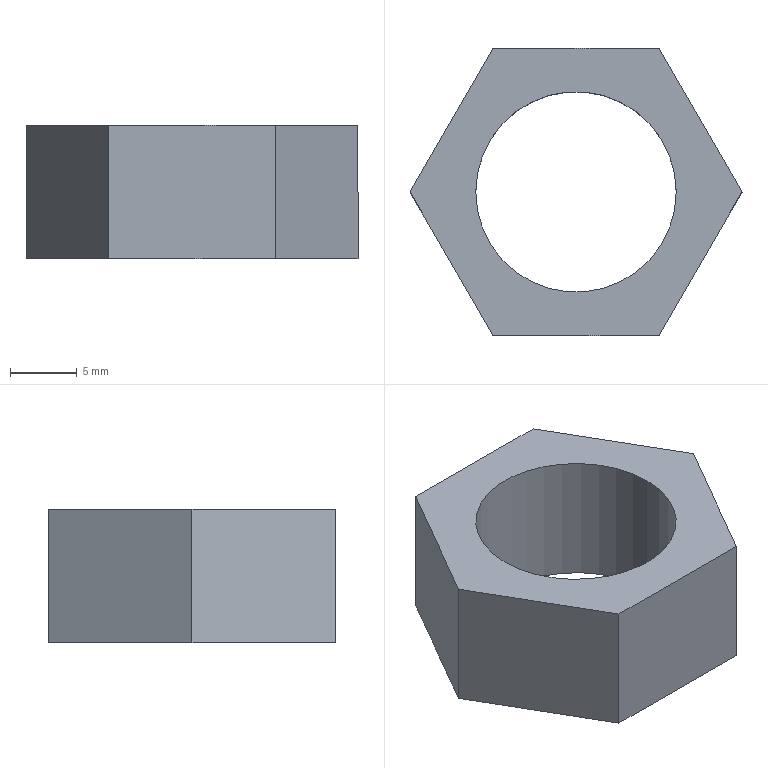Part | SolidWorks | features BaseBody 1 | 1 solid | 10 faces | box 24.848 x 21.519 x 10 mm | volume 2243 mm3 | plane 8 | cylinder 2 | commonest cylinder face diameters 15 x2
STEP:
#1=CARTESIAN_POINT('',(7.5,0.,0.));
#2=VERTEX_POINT('',#1);
#3=CARTESIAN_POINT('',(-7.5,0.,0.));
#4=VERTEX_POINT('',#3);
#5=CARTESIAN_POINT('',(0.,0.,0.));
#6=DIRECTION('',(0.,0.,-1.));
#7=DIRECTION('',(-1.,0.,0.));
#8=AXIS2_PLACEMENT_3D('',#5,#6,#7);
#9=CIRCLE('',#8,7.5);
#10=EDGE_CURVE('',#2,#4,#9,.T.);
#11=ORIENTED_EDGE('',*,*,#10,.F.);
#12=CARTESIAN_POINT('',(7.5,0.,-10.));
#13=VERTEX_POINT('',#12);
#14=CARTESIAN_POINT('',(7.5,0.,0.));
#15=DIRECTION('',(0.,0.,-1.));
#16=VECTOR('',#15,1000.);
#17=LINE('',#14,#16);
#18=EDGE_CURVE('',#2,#13,#17,.T.);
#19=ORIENTED_EDGE('',*,*,#18,.T.);
#20=CARTESIAN_POINT('',(-7.5,0.,-10.));
#21=VERTEX_POINT('',#20);
#22=CARTESIAN_POINT('',(0.,0.,-10.));
#23=DIRECTION('',(0.,0.,1.));
#24=DIRECTION('',(-1.,0.,0.));
#25=AXIS2_PLACEMENT_3D('',#22,#23,#24);
#26=CIRCLE('',#25,7.5);
#27=EDGE_CURVE('',#21,#13,#26,.T.);
#28=ORIENTED_EDGE('',*,*,#27,.F.);
#29=CARTESIAN_POINT('',(-7.5,0.,0.));
#30=DIRECTION('',(0.,0.,-1.));
#31=VECTOR('',#30,1000.);
#32=LINE('',#29,#31);
#33=EDGE_CURVE('',#4,#21,#32,.T.);
#34=ORIENTED_EDGE('',*,*,#33,.F.);
#35=EDGE_LOOP('',(#11,#19,#28,#34));
#36=FACE_OUTER_BOUND('',#35,.T.);
#37=CARTESIAN_POINT('',(0.,0.,0.));
#38=DIRECTION('',(0.,0.,-1.));
#39=DIRECTION('',(-1.,0.,0.));
#40=AXIS2_PLACEMENT_3D('',#37,#38,#39);
#41=CYLINDRICAL_SURFACE('',#40,7.5);
#42=ADVANCED_FACE('',(#36),#41,.F.);
#43=ORIENTED_EDGE('',*,*,#18,.F.);
#44=CARTESIAN_POINT('',(0.,0.,0.));
#45=DIRECTION('',(0.,0.,-1.));
#46=DIRECTION('',(-1.,0.,0.));
#47=AXIS2_PLACEMENT_3D('',#44,#45,#46);
#48=CIRCLE('',#47,7.5);
#49=EDGE_CURVE('',#4,#2,#48,.T.);
#50=ORIENTED_EDGE('',*,*,#49,.F.);
#51=ORIENTED_EDGE('',*,*,#33,.T.);
#52=CARTESIAN_POINT('',(0.,0.,-10.));
#53=DIRECTION('',(0.,0.,1.));
#54=DIRECTION('',(-1.,0.,0.));
#55=AXIS2_PLACEMENT_3D('',#52,#53,#54);
#56=CIRCLE('',#55,7.5);
#57=EDGE_CURVE('',#13,#21,#56,.T.);
#58=ORIENTED_EDGE('',*,*,#57,.F.);
#59=EDGE_LOOP('',(#43,#50,#51,#58));
#60=FACE_OUTER_BOUND('',#59,.T.);
#61=CARTESIAN_POINT('',(0.,0.,0.));
#62=DIRECTION('',(0.,0.,-1.));
#63=DIRECTION('',(-1.,0.,0.));
#64=AXIS2_PLACEMENT_3D('',#61,#62,#63);
#65=CYLINDRICAL_SURFACE('',#64,7.5);
#66=ADVANCED_FACE('',(#60),#65,.F.);
#67=ORIENTED_EDGE('',*,*,#27,.T.);
#68=ORIENTED_EDGE('',*,*,#57,.T.);
#69=EDGE_LOOP('',(#67,#68));
#70=FACE_BOUND('',#69,.T.);
#71=CARTESIAN_POINT('',(-6.212,-10.76,-10.));
#72=VERTEX_POINT('',#71);
#73=CARTESIAN_POINT('',(6.212,-10.76,-10.));
#74=VERTEX_POINT('',#73);
#75=CARTESIAN_POINT('',(0.,-10.76,-10.));
#76=DIRECTION('',(1.,0.,0.));
#77=VECTOR('',#76,1000.);
#78=LINE('',#75,#77);
#79=EDGE_CURVE('',#72,#74,#78,.T.);
#80=ORIENTED_EDGE('',*,*,#79,.F.);
#81=CARTESIAN_POINT('',(-12.424,0.,-10.));
#82=VERTEX_POINT('',#81);
#83=CARTESIAN_POINT('',(-12.424,0.,-10.));
#84=DIRECTION('',(0.5,-0.866,0.));
#85=VECTOR('',#84,1000.);
#86=LINE('',#83,#85);
#87=EDGE_CURVE('',#82,#72,#86,.T.);
#88=ORIENTED_EDGE('',*,*,#87,.F.);
#89=CARTESIAN_POINT('',(-6.212,10.76,-10.));
#90=VERTEX_POINT('',#89);
#91=CARTESIAN_POINT('',(-6.212,10.76,-10.));
#92=DIRECTION('',(-0.5,-0.866,0.));
#93=VECTOR('',#92,1000.);
#94=LINE('',#91,#93);
#95=EDGE_CURVE('',#90,#82,#94,.T.);
#96=ORIENTED_EDGE('',*,*,#95,.F.);
#97=CARTESIAN_POINT('',(6.212,10.76,-10.));
#98=VERTEX_POINT('',#97);
#99=CARTESIAN_POINT('',(0.,10.76,-10.));
#100=DIRECTION('',(-1.,0.,0.));
#101=VECTOR('',#100,1000.);
#102=LINE('',#99,#101);
#103=EDGE_CURVE('',#98,#90,#102,.T.);
#104=ORIENTED_EDGE('',*,*,#103,.F.);
#105=CARTESIAN_POINT('',(12.424,0.,-10.));
#106=VERTEX_POINT('',#105);
#107=CARTESIAN_POINT('',(12.424,0.,-10.));
#108=DIRECTION('',(-0.5,0.866,0.));
#109=VECTOR('',#108,1000.);
#110=LINE('',#107,#109);
#111=EDGE_CURVE('',#106,#98,#110,.T.);
#112=ORIENTED_EDGE('',*,*,#111,.F.);
#113=CARTESIAN_POINT('',(6.212,-10.76,-10.));
#114=DIRECTION('',(0.5,0.866,0.));
#115=VECTOR('',#114,1000.);
#116=LINE('',#113,#115);
#117=EDGE_CURVE('',#74,#106,#116,.T.);
#118=ORIENTED_EDGE('',*,*,#117,.F.);
#119=EDGE_LOOP('',(#80,#88,#96,#104,#112,#118));
#120=FACE_OUTER_BOUND('',#119,.T.);
#121=CARTESIAN_POINT('',(0.,0.,-10.));
#122=DIRECTION('',(0.,0.,1.));
#123=DIRECTION('',(1.,0.,0.));
#124=AXIS2_PLACEMENT_3D('',#121,#122,#123);
#125=PLANE('',#124);
#126=ADVANCED_FACE('',(#70,#120),#125,.F.);
#127=ORIENTED_EDGE('',*,*,#49,.T.);
#128=ORIENTED_EDGE('',*,*,#10,.T.);
#129=EDGE_LOOP('',(#127,#128));
#130=FACE_BOUND('',#129,.T.);
#131=CARTESIAN_POINT('',(-12.424,0.,0.));
#132=VERTEX_POINT('',#131);
#133=CARTESIAN_POINT('',(-6.212,-10.76,0.));
#134=VERTEX_POINT('',#133);
#135=CARTESIAN_POINT('',(-12.424,0.,0.));
#136=DIRECTION('',(0.5,-0.866,0.));
#137=VECTOR('',#136,1000.);
#138=LINE('',#135,#137);
#139=EDGE_CURVE('',#132,#134,#138,.T.);
#140=ORIENTED_EDGE('',*,*,#139,.T.);
#141=CARTESIAN_POINT('',(6.212,-10.76,0.));
#142=VERTEX_POINT('',#141);
#143=CARTESIAN_POINT('',(0.,-10.76,0.));
#144=DIRECTION('',(1.,0.,0.));
#145=VECTOR('',#144,1000.);
#146=LINE('',#143,#145);
#147=EDGE_CURVE('',#134,#142,#146,.T.);
#148=ORIENTED_EDGE('',*,*,#147,.T.);
#149=CARTESIAN_POINT('',(12.424,0.,0.));
#150=VERTEX_POINT('',#149);
#151=CARTESIAN_POINT('',(6.212,-10.76,0.));
#152=DIRECTION('',(0.5,0.866,0.));
#153=VECTOR('',#152,1000.);
#154=LINE('',#151,#153);
#155=EDGE_CURVE('',#142,#150,#154,.T.);
#156=ORIENTED_EDGE('',*,*,#155,.T.);
#157=CARTESIAN_POINT('',(6.212,10.76,0.));
#158=VERTEX_POINT('',#157);
#159=CARTESIAN_POINT('',(12.424,0.,0.));
#160=DIRECTION('',(-0.5,0.866,0.));
#161=VECTOR('',#160,1000.);
#162=LINE('',#159,#161);
#163=EDGE_CURVE('',#150,#158,#162,.T.);
#164=ORIENTED_EDGE('',*,*,#163,.T.);
#165=CARTESIAN_POINT('',(-6.212,10.76,0.));
#166=VERTEX_POINT('',#165);
#167=CARTESIAN_POINT('',(0.,10.76,0.));
#168=DIRECTION('',(-1.,0.,0.));
#169=VECTOR('',#168,1000.);
#170=LINE('',#167,#169);
#171=EDGE_CURVE('',#158,#166,#170,.T.);
#172=ORIENTED_EDGE('',*,*,#171,.T.);
#173=CARTESIAN_POINT('',(-6.212,10.76,0.));
#174=DIRECTION('',(-0.5,-0.866,0.));
#175=VECTOR('',#174,1000.);
#176=LINE('',#173,#175);
#177=EDGE_CURVE('',#166,#132,#176,.T.);
#178=ORIENTED_EDGE('',*,*,#177,.T.);
#179=EDGE_LOOP('',(#140,#148,#156,#164,#172,#178));
#180=FACE_OUTER_BOUND('',#179,.T.);
#181=CARTESIAN_POINT('',(0.,0.,0.));
#182=DIRECTION('',(0.,0.,1.));
#183=DIRECTION('',(1.,0.,0.));
#184=AXIS2_PLACEMENT_3D('',#181,#182,#183);
#185=PLANE('',#184);
#186=ADVANCED_FACE('',(#130,#180),#185,.T.);
#187=ORIENTED_EDGE('',*,*,#117,.T.);
#188=CARTESIAN_POINT('',(12.424,0.,0.));
#189=DIRECTION('',(0.,0.,1.));
#190=VECTOR('',#189,1000.);
#191=LINE('',#188,#190);
#192=EDGE_CURVE('',#106,#150,#191,.T.);
#193=ORIENTED_EDGE('',*,*,#192,.T.);
#194=ORIENTED_EDGE('',*,*,#155,.F.);
#195=CARTESIAN_POINT('',(6.212,-10.76,0.));
#196=DIRECTION('',(0.,0.,-1.));
#197=VECTOR('',#196,1000.);
#198=LINE('',#195,#197);
#199=EDGE_CURVE('',#142,#74,#198,.T.);
#200=ORIENTED_EDGE('',*,*,#199,.T.);
#201=EDGE_LOOP('',(#187,#193,#194,#200));
#202=FACE_OUTER_BOUND('',#201,.T.);
#203=CARTESIAN_POINT('',(12.424,0.,0.));
#204=DIRECTION('',(0.866,-0.5,0.));
#205=DIRECTION('',(0.5,0.866,0.));
#206=AXIS2_PLACEMENT_3D('',#203,#204,#205);
#207=PLANE('',#206);
#208=ADVANCED_FACE('',(#202),#207,.T.);
#209=ORIENTED_EDGE('',*,*,#79,.T.);
#210=ORIENTED_EDGE('',*,*,#199,.F.);
#211=ORIENTED_EDGE('',*,*,#147,.F.);
#212=CARTESIAN_POINT('',(-6.212,-10.76,0.));
#213=DIRECTION('',(0.,0.,-1.));
#214=VECTOR('',#213,1000.);
#215=LINE('',#212,#214);
#216=EDGE_CURVE('',#134,#72,#215,.T.);
#217=ORIENTED_EDGE('',*,*,#216,.T.);
#218=EDGE_LOOP('',(#209,#210,#211,#217));
#219=FACE_OUTER_BOUND('',#218,.T.);
#220=CARTESIAN_POINT('',(6.212,-10.76,0.));
#221=DIRECTION('',(0.,-1.,0.));
#222=DIRECTION('',(0.,0.,-1.));
#223=AXIS2_PLACEMENT_3D('',#220,#221,#222);
#224=PLANE('',#223);
#225=ADVANCED_FACE('',(#219),#224,.T.);
#226=ORIENTED_EDGE('',*,*,#87,.T.);
#227=ORIENTED_EDGE('',*,*,#216,.F.);
#228=ORIENTED_EDGE('',*,*,#139,.F.);
#229=CARTESIAN_POINT('',(-12.424,0.,0.));
#230=DIRECTION('',(0.,0.,-1.));
#231=VECTOR('',#230,1000.);
#232=LINE('',#229,#231);
#233=EDGE_CURVE('',#132,#82,#232,.T.);
#234=ORIENTED_EDGE('',*,*,#233,.T.);
#235=EDGE_LOOP('',(#226,#227,#228,#234));
#236=FACE_OUTER_BOUND('',#235,.T.);
#237=CARTESIAN_POINT('',(-6.212,-10.76,0.));
#238=DIRECTION('',(-0.866,-0.5,0.));
#239=DIRECTION('',(0.5,-0.866,0.));
#240=AXIS2_PLACEMENT_3D('',#237,#238,#239);
#241=PLANE('',#240);
#242=ADVANCED_FACE('',(#236),#241,.T.);
#243=ORIENTED_EDGE('',*,*,#95,.T.);
#244=ORIENTED_EDGE('',*,*,#233,.F.);
#245=ORIENTED_EDGE('',*,*,#177,.F.);
#246=CARTESIAN_POINT('',(-6.212,10.76,0.));
#247=DIRECTION('',(0.,0.,-1.));
#248=VECTOR('',#247,1000.);
#249=LINE('',#246,#248);
#250=EDGE_CURVE('',#166,#90,#249,.T.);
#251=ORIENTED_EDGE('',*,*,#250,.T.);
#252=EDGE_LOOP('',(#243,#244,#245,#251));
#253=FACE_OUTER_BOUND('',#252,.T.);
#254=CARTESIAN_POINT('',(-12.424,0.,0.));
#255=DIRECTION('',(-0.866,0.5,0.));
#256=DIRECTION('',(-0.5,-0.866,0.));
#257=AXIS2_PLACEMENT_3D('',#254,#255,#256);
#258=PLANE('',#257);
#259=ADVANCED_FACE('',(#253),#258,.T.);
#260=ORIENTED_EDGE('',*,*,#103,.T.);
#261=ORIENTED_EDGE('',*,*,#250,.F.);
#262=ORIENTED_EDGE('',*,*,#171,.F.);
#263=CARTESIAN_POINT('',(6.212,10.76,0.));
#264=DIRECTION('',(0.,0.,-1.));
#265=VECTOR('',#264,1000.);
#266=LINE('',#263,#265);
#267=EDGE_CURVE('',#158,#98,#266,.T.);
#268=ORIENTED_EDGE('',*,*,#267,.T.);
#269=EDGE_LOOP('',(#260,#261,#262,#268));
#270=FACE_OUTER_BOUND('',#269,.T.);
#271=CARTESIAN_POINT('',(-6.212,10.76,0.));
#272=DIRECTION('',(0.,1.,0.));
#273=DIRECTION('',(-1.,0.,0.));
#274=AXIS2_PLACEMENT_3D('',#271,#272,#273);
#275=PLANE('',#274);
#276=ADVANCED_FACE('',(#270),#275,.T.);
#277=ORIENTED_EDGE('',*,*,#111,.T.);
#278=ORIENTED_EDGE('',*,*,#267,.F.);
#279=ORIENTED_EDGE('',*,*,#163,.F.);
#280=ORIENTED_EDGE('',*,*,#192,.F.);
#281=EDGE_LOOP('',(#277,#278,#279,#280));
#282=FACE_OUTER_BOUND('',#281,.T.);
#283=CARTESIAN_POINT('',(6.212,10.76,0.));
#284=DIRECTION('',(0.866,0.5,0.));
#285=DIRECTION('',(-0.5,0.866,0.));
#286=AXIS2_PLACEMENT_3D('',#283,#284,#285);
#287=PLANE('',#286);
#288=ADVANCED_FACE('',(#282),#287,.T.);
#289=CLOSED_SHELL('',(#42,#66,#126,#186,#208,#225,#242,#259,#276,#288));
#290=MANIFOLD_SOLID_BREP('',#289);
#291=CARTESIAN_POINT('',(0.,0.,0.));
#292=DIRECTION('',(0.,0.,1.));
#293=DIRECTION('',(1.,0.,0.));
#294=AXIS2_PLACEMENT_3D('',#291,#292,#293);
#295=(LENGTH_UNIT()NAMED_UNIT(*)SI_UNIT(.MILLI.,.METRE.));
#296=UNCERTAINTY_MEASURE_WITH_UNIT(LENGTH_MEASURE(0.00001),#295,'','');
#297=(NAMED_UNIT(*)PLANE_ANGLE_UNIT()SI_UNIT($,.RADIAN.));
#298=(NAMED_UNIT(*)SI_UNIT($,.STERADIAN.)SOLID_ANGLE_UNIT());
#299=(GEOMETRIC_REPRESENTATION_CONTEXT(3)GLOBAL_UNCERTAINTY_ASSIGNED_CONTEXT((#296))GLOBAL_UNIT_ASSIGNED_CONTEXT((#295,#297,#298))REPRESENTATION_CONTEXT('',''));
#300=ADVANCED_BREP_SHAPE_REPRESENTATION('',(#290,#294),#299);